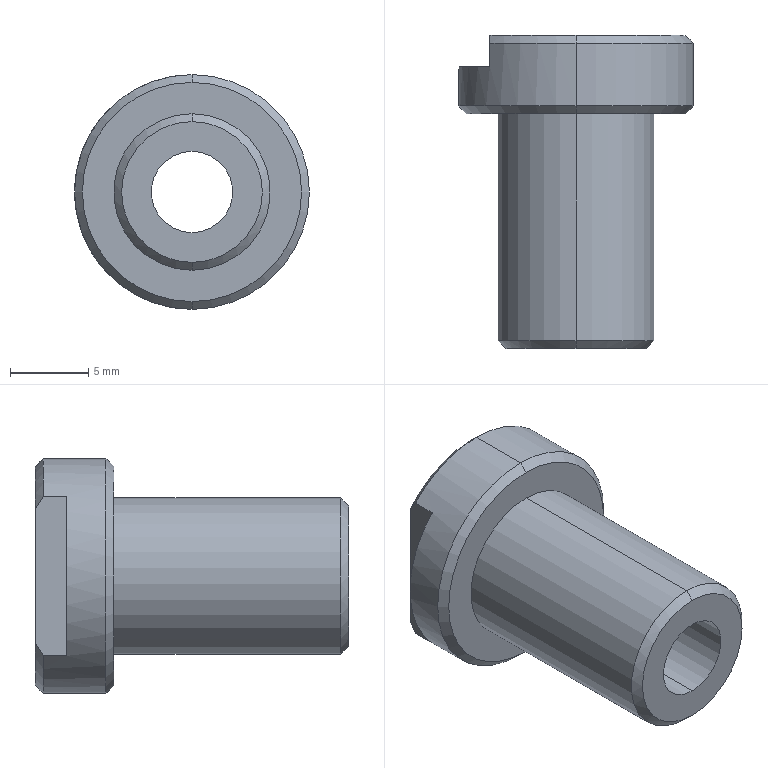Part | SolidWorks | features ICE 2, Chamfer 1, Extrusion 1 | 1 solid | 20 faces | box 15 x 20 x 15 mm | volume 1593 mm3 | cone 9 | cylinder 6 | plane 5 | commonest cylinder face diameters 5.2 x2 10 x2 15 x2
STEP:
#1=CARTESIAN_POINT('',(0.,0.,-4.5));
#2=VERTEX_POINT('',#1);
#3=CARTESIAN_POINT('',(0.,0.,4.5));
#4=VERTEX_POINT('',#3);
#5=CARTESIAN_POINT('',(0.,0.,0.));
#6=DIRECTION('',(0.,-1.,0.));
#7=DIRECTION('',(0.,0.,1.));
#8=AXIS2_PLACEMENT_3D('',#5,#6,#7);
#9=CIRCLE('',#8,4.5);
#10=EDGE_CURVE('',#2,#4,#9,.T.);
#11=ORIENTED_EDGE('',*,*,#10,.F.);
#12=CARTESIAN_POINT('',(0.,0.5,-5.));
#13=VERTEX_POINT('',#12);
#14=CARTESIAN_POINT('',(0.,0.5,-5.));
#15=DIRECTION('',(0.,0.7071,-0.7071));
#16=VECTOR('',#15,1000.);
#17=LINE('',#14,#16);
#18=EDGE_CURVE('',#2,#13,#17,.T.);
#19=ORIENTED_EDGE('',*,*,#18,.T.);
#20=CARTESIAN_POINT('',(0.,0.5,5.));
#21=VERTEX_POINT('',#20);
#22=CARTESIAN_POINT('',(0.,0.5,0.));
#23=DIRECTION('',(0.,1.,0.));
#24=DIRECTION('',(0.,0.,1.));
#25=AXIS2_PLACEMENT_3D('',#22,#23,#24);
#26=CIRCLE('',#25,5.);
#27=EDGE_CURVE('',#21,#13,#26,.T.);
#28=ORIENTED_EDGE('',*,*,#27,.F.);
#29=CARTESIAN_POINT('',(0.,0.5,5.));
#30=DIRECTION('',(0.,0.7071,0.7071));
#31=VECTOR('',#30,1000.);
#32=LINE('',#29,#31);
#33=EDGE_CURVE('',#4,#21,#32,.T.);
#34=ORIENTED_EDGE('',*,*,#33,.F.);
#35=EDGE_LOOP('',(#11,#19,#28,#34));
#36=FACE_OUTER_BOUND('',#35,.T.);
#37=CARTESIAN_POINT('',(0.,0.5,0.));
#38=DIRECTION('',(0.,1.,0.));
#39=DIRECTION('',(0.,0.,1.));
#40=AXIS2_PLACEMENT_3D('',#37,#38,#39);
#41=CONICAL_SURFACE('',#40,5.,0.7854);
#42=ADVANCED_FACE('',(#36),#41,.T.);
#43=CARTESIAN_POINT('',(0.,19.5,-2.6));
#44=VERTEX_POINT('',#43);
#45=CARTESIAN_POINT('',(0.,19.5,2.6));
#46=VERTEX_POINT('',#45);
#47=CARTESIAN_POINT('',(0.,19.5,0.));
#48=DIRECTION('',(0.,1.,0.));
#49=DIRECTION('',(0.,0.,1.));
#50=AXIS2_PLACEMENT_3D('',#47,#48,#49);
#51=CIRCLE('',#50,2.6);
#52=EDGE_CURVE('',#44,#46,#51,.T.);
#53=ORIENTED_EDGE('',*,*,#52,.F.);
#54=CARTESIAN_POINT('',(0.,20.,-3.1));
#55=VERTEX_POINT('',#54);
#56=CARTESIAN_POINT('',(0.,19.5,-2.6));
#57=DIRECTION('',(0.,0.7071,-0.7071));
#58=VECTOR('',#57,1000.);
#59=LINE('',#56,#58);
#60=EDGE_CURVE('',#44,#55,#59,.T.);
#61=ORIENTED_EDGE('',*,*,#60,.T.);
#62=CARTESIAN_POINT('',(0.,20.,3.1));
#63=VERTEX_POINT('',#62);
#64=CARTESIAN_POINT('',(0.,20.,0.));
#65=DIRECTION('',(0.,-1.,0.));
#66=DIRECTION('',(0.,0.,1.));
#67=AXIS2_PLACEMENT_3D('',#64,#65,#66);
#68=CIRCLE('',#67,3.1);
#69=EDGE_CURVE('',#63,#55,#68,.T.);
#70=ORIENTED_EDGE('',*,*,#69,.F.);
#71=CARTESIAN_POINT('',(0.,19.5,2.6));
#72=DIRECTION('',(0.,0.7071,0.7071));
#73=VECTOR('',#72,1000.);
#74=LINE('',#71,#73);
#75=EDGE_CURVE('',#46,#63,#74,.T.);
#76=ORIENTED_EDGE('',*,*,#75,.F.);
#77=EDGE_LOOP('',(#53,#61,#70,#76));
#78=FACE_OUTER_BOUND('',#77,.T.);
#79=CARTESIAN_POINT('',(0.,19.5,0.));
#80=DIRECTION('',(0.,1.,0.));
#81=DIRECTION('',(0.,0.,1.));
#82=AXIS2_PLACEMENT_3D('',#79,#80,#81);
#83=CONICAL_SURFACE('',#82,2.6,0.7854);
#84=ADVANCED_FACE('',(#78),#83,.F.);
#85=CARTESIAN_POINT('',(0.,20.,7.));
#86=VERTEX_POINT('',#85);
#87=CARTESIAN_POINT('',(0.,20.,-7.));
#88=VERTEX_POINT('',#87);
#89=CARTESIAN_POINT('',(0.,20.,0.));
#90=DIRECTION('',(0.,1.,0.));
#91=DIRECTION('',(0.,0.,1.));
#92=AXIS2_PLACEMENT_3D('',#89,#90,#91);
#93=CIRCLE('',#92,7.);
#94=EDGE_CURVE('',#86,#88,#93,.T.);
#95=ORIENTED_EDGE('',*,*,#94,.F.);
#96=CARTESIAN_POINT('',(0.,19.5,7.5));
#97=VERTEX_POINT('',#96);
#98=CARTESIAN_POINT('',(0.,20.,7.));
#99=DIRECTION('',(0.,-0.7071,0.7071));
#100=VECTOR('',#99,1000.);
#101=LINE('',#98,#100);
#102=EDGE_CURVE('',#86,#97,#101,.T.);
#103=ORIENTED_EDGE('',*,*,#102,.T.);
#104=CARTESIAN_POINT('',(0.,19.5,-7.5));
#105=VERTEX_POINT('',#104);
#106=CARTESIAN_POINT('',(0.,19.5,0.));
#107=DIRECTION('',(0.,-1.,0.));
#108=DIRECTION('',(0.,0.,1.));
#109=AXIS2_PLACEMENT_3D('',#106,#107,#108);
#110=CIRCLE('',#109,7.5);
#111=EDGE_CURVE('',#105,#97,#110,.T.);
#112=ORIENTED_EDGE('',*,*,#111,.F.);
#113=CARTESIAN_POINT('',(0.,20.,-7.));
#114=DIRECTION('',(0.,-0.7071,-0.7071));
#115=VECTOR('',#114,1000.);
#116=LINE('',#113,#115);
#117=EDGE_CURVE('',#88,#105,#116,.T.);
#118=ORIENTED_EDGE('',*,*,#117,.F.);
#119=EDGE_LOOP('',(#95,#103,#112,#118));
#120=FACE_OUTER_BOUND('',#119,.T.);
#121=CARTESIAN_POINT('',(0.,20.,0.));
#122=DIRECTION('',(0.,-1.,0.));
#123=DIRECTION('',(0.,0.,-1.));
#124=AXIS2_PLACEMENT_3D('',#121,#122,#123);
#125=CONICAL_SURFACE('',#124,7.,0.7854);
#126=ADVANCED_FACE('',(#120),#125,.T.);
#127=CARTESIAN_POINT('',(-5.5,20.,-4.33));
#128=VERTEX_POINT('',#127);
#129=CARTESIAN_POINT('',(0.,20.,0.));
#130=DIRECTION('',(0.,1.,0.));
#131=DIRECTION('',(0.,0.,1.));
#132=AXIS2_PLACEMENT_3D('',#129,#130,#131);
#133=CIRCLE('',#132,7.);
#134=EDGE_CURVE('',#88,#128,#133,.T.);
#135=ORIENTED_EDGE('',*,*,#134,.F.);
#136=ORIENTED_EDGE('',*,*,#117,.T.);
#137=CARTESIAN_POINT('',(-5.5,19.5,-5.099));
#138=VERTEX_POINT('',#137);
#139=CARTESIAN_POINT('',(0.,19.5,0.));
#140=DIRECTION('',(0.,-1.,0.));
#141=DIRECTION('',(0.,0.,1.));
#142=AXIS2_PLACEMENT_3D('',#139,#140,#141);
#143=CIRCLE('',#142,7.5);
#144=EDGE_CURVE('',#138,#105,#143,.T.);
#145=ORIENTED_EDGE('',*,*,#144,.F.);
#146=CARTESIAN_POINT('',(-5.5,20.,-4.33));
#147=CARTESIAN_POINT('',(-5.5,19.839,-4.59));
#148=CARTESIAN_POINT('',(-5.5,19.672,-4.846));
#149=CARTESIAN_POINT('',(-5.5,19.5,-5.099));
#150=B_SPLINE_CURVE_WITH_KNOTS('',3,(#146,#147,#148,#149),.UNSPECIFIED.,.F.,.F.,(4,4),(0.01014,0.01105),.UNSPECIFIED.);
#151=EDGE_CURVE('',#128,#138,#150,.T.);
#152=ORIENTED_EDGE('',*,*,#151,.F.);
#153=EDGE_LOOP('',(#135,#136,#145,#152));
#154=FACE_OUTER_BOUND('',#153,.T.);
#155=CARTESIAN_POINT('',(0.,20.,0.));
#156=DIRECTION('',(0.,-1.,0.));
#157=DIRECTION('',(0.,0.,-1.));
#158=AXIS2_PLACEMENT_3D('',#155,#156,#157);
#159=CONICAL_SURFACE('',#158,7.,0.7854);
#160=ADVANCED_FACE('',(#154),#159,.T.);
#161=CARTESIAN_POINT('',(0.,15.,-7.));
#162=VERTEX_POINT('',#161);
#163=CARTESIAN_POINT('',(0.,15.,7.));
#164=VERTEX_POINT('',#163);
#165=CARTESIAN_POINT('',(0.,15.,0.));
#166=DIRECTION('',(0.,-1.,0.));
#167=DIRECTION('',(0.,0.,1.));
#168=AXIS2_PLACEMENT_3D('',#165,#166,#167);
#169=CIRCLE('',#168,7.);
#170=EDGE_CURVE('',#162,#164,#169,.T.);
#171=ORIENTED_EDGE('',*,*,#170,.F.);
#172=CARTESIAN_POINT('',(0.,15.5,-7.5));
#173=VERTEX_POINT('',#172);
#174=CARTESIAN_POINT('',(0.,15.5,-7.5));
#175=DIRECTION('',(0.,0.7071,-0.7071));
#176=VECTOR('',#175,1000.);
#177=LINE('',#174,#176);
#178=EDGE_CURVE('',#162,#173,#177,.T.);
#179=ORIENTED_EDGE('',*,*,#178,.T.);
#180=CARTESIAN_POINT('',(0.,15.5,7.5));
#181=VERTEX_POINT('',#180);
#182=CARTESIAN_POINT('',(0.,15.5,0.));
#183=DIRECTION('',(0.,1.,0.));
#184=DIRECTION('',(0.,0.,1.));
#185=AXIS2_PLACEMENT_3D('',#182,#183,#184);
#186=CIRCLE('',#185,7.5);
#187=EDGE_CURVE('',#181,#173,#186,.T.);
#188=ORIENTED_EDGE('',*,*,#187,.F.);
#189=CARTESIAN_POINT('',(0.,15.5,7.5));
#190=DIRECTION('',(0.,0.7071,0.7071));
#191=VECTOR('',#190,1000.);
#192=LINE('',#189,#191);
#193=EDGE_CURVE('',#164,#181,#192,.T.);
#194=ORIENTED_EDGE('',*,*,#193,.F.);
#195=EDGE_LOOP('',(#171,#179,#188,#194));
#196=FACE_OUTER_BOUND('',#195,.T.);
#197=CARTESIAN_POINT('',(0.,15.5,0.));
#198=DIRECTION('',(0.,1.,0.));
#199=DIRECTION('',(0.,0.,1.));
#200=AXIS2_PLACEMENT_3D('',#197,#198,#199);
#201=CONICAL_SURFACE('',#200,7.5,0.7854);
#202=ADVANCED_FACE('',(#196),#201,.T.);
#203=ORIENTED_EDGE('',*,*,#111,.T.);
#204=CARTESIAN_POINT('',(0.,20.,7.5));
#205=DIRECTION('',(0.,-1.,0.));
#206=VECTOR('',#205,1000.);
#207=LINE('',#204,#206);
#208=EDGE_CURVE('',#97,#181,#207,.T.);
#209=ORIENTED_EDGE('',*,*,#208,.T.);
#210=ORIENTED_EDGE('',*,*,#187,.T.);
#211=CARTESIAN_POINT('',(0.,20.,-7.5));
#212=DIRECTION('',(0.,-1.,0.));
#213=VECTOR('',#212,1000.);
#214=LINE('',#211,#213);
#215=EDGE_CURVE('',#105,#173,#214,.T.);
#216=ORIENTED_EDGE('',*,*,#215,.F.);
#217=EDGE_LOOP('',(#203,#209,#210,#216));
#218=FACE_OUTER_BOUND('',#217,.T.);
#219=CARTESIAN_POINT('',(0.,20.,0.));
#220=DIRECTION('',(0.,-1.,0.));
#221=DIRECTION('',(0.,0.,-1.));
#222=AXIS2_PLACEMENT_3D('',#219,#220,#221);
#223=CYLINDRICAL_SURFACE('',#222,7.5);
#224=ADVANCED_FACE('',(#218),#223,.T.);
#225=ORIENTED_EDGE('',*,*,#52,.T.);
#226=CARTESIAN_POINT('',(0.,0.,2.6));
#227=VERTEX_POINT('',#226);
#228=CARTESIAN_POINT('',(0.,15.,2.6));
#229=DIRECTION('',(0.,-1.,0.));
#230=VECTOR('',#229,1000.);
#231=LINE('',#228,#230);
#232=EDGE_CURVE('',#46,#227,#231,.T.);
#233=ORIENTED_EDGE('',*,*,#232,.T.);
#234=CARTESIAN_POINT('',(0.,0.,-2.6));
#235=VERTEX_POINT('',#234);
#236=CARTESIAN_POINT('',(0.,0.,0.));
#237=DIRECTION('',(0.,1.,0.));
#238=DIRECTION('',(0.,0.,1.));
#239=AXIS2_PLACEMENT_3D('',#236,#237,#238);
#240=CIRCLE('',#239,2.6);
#241=EDGE_CURVE('',#235,#227,#240,.T.);
#242=ORIENTED_EDGE('',*,*,#241,.F.);
#243=CARTESIAN_POINT('',(0.,15.,-2.6));
#244=DIRECTION('',(0.,-1.,0.));
#245=VECTOR('',#244,1000.);
#246=LINE('',#243,#245);
#247=EDGE_CURVE('',#44,#235,#246,.T.);
#248=ORIENTED_EDGE('',*,*,#247,.F.);
#249=EDGE_LOOP('',(#225,#233,#242,#248));
#250=FACE_OUTER_BOUND('',#249,.T.);
#251=CARTESIAN_POINT('',(0.,15.,0.));
#252=DIRECTION('',(0.,-1.,0.));
#253=DIRECTION('',(0.,0.,-1.));
#254=AXIS2_PLACEMENT_3D('',#251,#252,#253);
#255=CYLINDRICAL_SURFACE('',#254,2.6);
#256=ADVANCED_FACE('',(#250),#255,.F.);
#257=CARTESIAN_POINT('',(0.,15.,5.));
#258=VERTEX_POINT('',#257);
#259=CARTESIAN_POINT('',(0.,15.,-5.));
#260=VERTEX_POINT('',#259);
#261=CARTESIAN_POINT('',(0.,15.,0.));
#262=DIRECTION('',(0.,1.,0.));
#263=DIRECTION('',(0.,0.,1.));
#264=AXIS2_PLACEMENT_3D('',#261,#262,#263);
#265=CIRCLE('',#264,5.);
#266=EDGE_CURVE('',#258,#260,#265,.T.);
#267=ORIENTED_EDGE('',*,*,#266,.F.);
#268=CARTESIAN_POINT('',(0.,15.,5.));
#269=DIRECTION('',(0.,-1.,0.));
#270=VECTOR('',#269,1000.);
#271=LINE('',#268,#270);
#272=EDGE_CURVE('',#258,#21,#271,.T.);
#273=ORIENTED_EDGE('',*,*,#272,.T.);
#274=ORIENTED_EDGE('',*,*,#27,.T.);
#275=CARTESIAN_POINT('',(0.,15.,-5.));
#276=DIRECTION('',(0.,-1.,0.));
#277=VECTOR('',#276,1000.);
#278=LINE('',#275,#277);
#279=EDGE_CURVE('',#260,#13,#278,.T.);
#280=ORIENTED_EDGE('',*,*,#279,.F.);
#281=EDGE_LOOP('',(#267,#273,#274,#280));
#282=FACE_OUTER_BOUND('',#281,.T.);
#283=CARTESIAN_POINT('',(0.,15.,0.));
#284=DIRECTION('',(0.,-1.,0.));
#285=DIRECTION('',(0.,0.,-1.));
#286=AXIS2_PLACEMENT_3D('',#283,#284,#285);
#287=CYLINDRICAL_SURFACE('',#286,5.);
#288=ADVANCED_FACE('',(#282),#287,.T.);
#289=CARTESIAN_POINT('',(0.,0.,0.));
#290=DIRECTION('',(0.,-1.,0.));
#291=DIRECTION('',(0.,0.,1.));
#292=AXIS2_PLACEMENT_3D('',#289,#290,#291);
#293=CIRCLE('',#292,4.5);
#294=EDGE_CURVE('',#4,#2,#293,.T.);
#295=ORIENTED_EDGE('',*,*,#294,.T.);
#296=ORIENTED_EDGE('',*,*,#10,.T.);
#297=EDGE_LOOP('',(#295,#296));
#298=FACE_OUTER_BOUND('',#297,.T.);
#299=ORIENTED_EDGE('',*,*,#241,.T.);
#300=CARTESIAN_POINT('',(0.,0.,0.));
#301=DIRECTION('',(0.,1.,0.));
#302=DIRECTION('',(0.,0.,1.));
#303=AXIS2_PLACEMENT_3D('',#300,#301,#302);
#304=CIRCLE('',#303,2.6);
#305=EDGE_CURVE('',#227,#235,#304,.T.);
#306=ORIENTED_EDGE('',*,*,#305,.T.);
#307=EDGE_LOOP('',(#299,#306));
#308=FACE_BOUND('',#307,.T.);
#309=CARTESIAN_POINT('',(0.,0.,0.));
#310=DIRECTION('',(0.,1.,0.));
#311=DIRECTION('',(0.,0.,1.));
#312=AXIS2_PLACEMENT_3D('',#309,#310,#311);
#313=PLANE('',#312);
#314=ADVANCED_FACE('',(#298,#308),#313,.F.);
#315=ORIENTED_EDGE('',*,*,#272,.F.);
#316=CARTESIAN_POINT('',(0.,15.,0.));
#317=DIRECTION('',(0.,1.,0.));
#318=DIRECTION('',(0.,0.,1.));
#319=AXIS2_PLACEMENT_3D('',#316,#317,#318);
#320=CIRCLE('',#319,5.);
#321=EDGE_CURVE('',#260,#258,#320,.T.);
#322=ORIENTED_EDGE('',*,*,#321,.F.);
#323=ORIENTED_EDGE('',*,*,#279,.T.);
#324=CARTESIAN_POINT('',(0.,0.5,0.));
#325=DIRECTION('',(0.,1.,0.));
#326=DIRECTION('',(0.,0.,1.));
#327=AXIS2_PLACEMENT_3D('',#324,#325,#326);
#328=CIRCLE('',#327,5.);
#329=EDGE_CURVE('',#13,#21,#328,.T.);
#330=ORIENTED_EDGE('',*,*,#329,.T.);
#331=EDGE_LOOP('',(#315,#322,#323,#330));
#332=FACE_OUTER_BOUND('',#331,.T.);
#333=CARTESIAN_POINT('',(0.,15.,0.));
#334=DIRECTION('',(0.,-1.,0.));
#335=DIRECTION('',(0.,0.,-1.));
#336=AXIS2_PLACEMENT_3D('',#333,#334,#335);
#337=CYLINDRICAL_SURFACE('',#336,5.);
#338=ADVANCED_FACE('',(#332),#337,.T.);
#339=ORIENTED_EDGE('',*,*,#232,.F.);
#340=CARTESIAN_POINT('',(0.,19.5,0.));
#341=DIRECTION('',(0.,1.,0.));
#342=DIRECTION('',(0.,0.,1.));
#343=AXIS2_PLACEMENT_3D('',#340,#341,#342);
#344=CIRCLE('',#343,2.6);
#345=EDGE_CURVE('',#46,#44,#344,.T.);
#346=ORIENTED_EDGE('',*,*,#345,.T.);
#347=ORIENTED_EDGE('',*,*,#247,.T.);
#348=ORIENTED_EDGE('',*,*,#305,.F.);
#349=EDGE_LOOP('',(#339,#346,#347,#348));
#350=FACE_OUTER_BOUND('',#349,.T.);
#351=CARTESIAN_POINT('',(0.,15.,0.));
#352=DIRECTION('',(0.,-1.,0.));
#353=DIRECTION('',(0.,0.,-1.));
#354=AXIS2_PLACEMENT_3D('',#351,#352,#353);
#355=CYLINDRICAL_SURFACE('',#354,2.6);
#356=ADVANCED_FACE('',(#350),#355,.F.);
#357=CARTESIAN_POINT('',(-5.5,20.,4.33));
#358=VERTEX_POINT('',#357);
#359=CARTESIAN_POINT('',(-5.5,20.,0.));
#360=DIRECTION('',(0.,0.,-1.));
#361=VECTOR('',#360,1000.);
#362=LINE('',#359,#361);
#363=EDGE_CURVE('',#358,#128,#362,.T.);
#364=ORIENTED_EDGE('',*,*,#363,.F.);
#365=CARTESIAN_POINT('',(0.,20.,0.));
#366=DIRECTION('',(0.,1.,0.));
#367=DIRECTION('',(0.,0.,1.));
#368=AXIS2_PLACEMENT_3D('',#365,#366,#367);
#369=CIRCLE('',#368,7.);
#370=EDGE_CURVE('',#358,#86,#369,.T.);
#371=ORIENTED_EDGE('',*,*,#370,.T.);
#372=ORIENTED_EDGE('',*,*,#94,.T.);
#373=ORIENTED_EDGE('',*,*,#134,.T.);
#374=EDGE_LOOP('',(#364,#371,#372,#373));
#375=FACE_OUTER_BOUND('',#374,.T.);
#376=ORIENTED_EDGE('',*,*,#69,.T.);
#377=CARTESIAN_POINT('',(0.,20.,0.));
#378=DIRECTION('',(0.,-1.,0.));
#379=DIRECTION('',(0.,0.,1.));
#380=AXIS2_PLACEMENT_3D('',#377,#378,#379);
#381=CIRCLE('',#380,3.1);
#382=EDGE_CURVE('',#55,#63,#381,.T.);
#383=ORIENTED_EDGE('',*,*,#382,.T.);
#384=EDGE_LOOP('',(#376,#383));
#385=FACE_BOUND('',#384,.T.);
#386=CARTESIAN_POINT('',(0.,20.,0.));
#387=DIRECTION('',(0.,1.,0.));
#388=DIRECTION('',(0.,0.,1.));
#389=AXIS2_PLACEMENT_3D('',#386,#387,#388);
#390=PLANE('',#389);
#391=ADVANCED_FACE('',(#375,#385),#390,.T.);
#392=CARTESIAN_POINT('',(0.,15.,0.));
#393=DIRECTION('',(0.,-1.,0.));
#394=DIRECTION('',(0.,0.,1.));
#395=AXIS2_PLACEMENT_3D('',#392,#393,#394);
#396=CIRCLE('',#395,7.);
#397=EDGE_CURVE('',#164,#162,#396,.T.);
#398=ORIENTED_EDGE('',*,*,#397,.T.);
#399=ORIENTED_EDGE('',*,*,#170,.T.);
#400=EDGE_LOOP('',(#398,#399));
#401=FACE_OUTER_BOUND('',#400,.T.);
#402=ORIENTED_EDGE('',*,*,#321,.T.);
#403=ORIENTED_EDGE('',*,*,#266,.T.);
#404=EDGE_LOOP('',(#402,#403));
#405=FACE_BOUND('',#404,.T.);
#406=CARTESIAN_POINT('',(0.,15.,0.));
#407=DIRECTION('',(0.,1.,0.));
#408=DIRECTION('',(0.,0.,1.));
#409=AXIS2_PLACEMENT_3D('',#406,#407,#408);
#410=PLANE('',#409);
#411=ADVANCED_FACE('',(#401,#405),#410,.F.);
#412=ORIENTED_EDGE('',*,*,#208,.F.);
#413=CARTESIAN_POINT('',(-5.5,19.5,5.099));
#414=VERTEX_POINT('',#413);
#415=CARTESIAN_POINT('',(0.,19.5,0.));
#416=DIRECTION('',(0.,-1.,0.));
#417=DIRECTION('',(0.,0.,1.));
#418=AXIS2_PLACEMENT_3D('',#415,#416,#417);
#419=CIRCLE('',#418,7.5);
#420=EDGE_CURVE('',#97,#414,#419,.T.);
#421=ORIENTED_EDGE('',*,*,#420,.T.);
#422=CARTESIAN_POINT('',(-5.5,18.,5.099));
#423=VERTEX_POINT('',#422);
#424=CARTESIAN_POINT('',(-5.5,20.,5.099));
#425=DIRECTION('',(0.,-1.,0.));
#426=VECTOR('',#425,1000.);
#427=LINE('',#424,#426);
#428=EDGE_CURVE('',#414,#423,#427,.T.);
#429=ORIENTED_EDGE('',*,*,#428,.T.);
#430=CARTESIAN_POINT('',(-5.5,18.,-5.099));
#431=VERTEX_POINT('',#430);
#432=CARTESIAN_POINT('',(0.,18.,0.));
#433=DIRECTION('',(0.,-1.,0.));
#434=DIRECTION('',(0.,0.,-1.));
#435=AXIS2_PLACEMENT_3D('',#432,#433,#434);
#436=CIRCLE('',#435,7.5);
#437=EDGE_CURVE('',#423,#431,#436,.T.);
#438=ORIENTED_EDGE('',*,*,#437,.T.);
#439=CARTESIAN_POINT('',(-5.5,20.,-5.099));
#440=DIRECTION('',(0.,1.,0.));
#441=VECTOR('',#440,1000.);
#442=LINE('',#439,#441);
#443=EDGE_CURVE('',#431,#138,#442,.T.);
#444=ORIENTED_EDGE('',*,*,#443,.T.);
#445=ORIENTED_EDGE('',*,*,#144,.T.);
#446=ORIENTED_EDGE('',*,*,#215,.T.);
#447=CARTESIAN_POINT('',(0.,15.5,0.));
#448=DIRECTION('',(0.,1.,0.));
#449=DIRECTION('',(0.,0.,1.));
#450=AXIS2_PLACEMENT_3D('',#447,#448,#449);
#451=CIRCLE('',#450,7.5);
#452=EDGE_CURVE('',#173,#181,#451,.T.);
#453=ORIENTED_EDGE('',*,*,#452,.T.);
#454=EDGE_LOOP('',(#412,#421,#429,#438,#444,#445,#446,#453));
#455=FACE_OUTER_BOUND('',#454,.T.);
#456=CARTESIAN_POINT('',(0.,20.,0.));
#457=DIRECTION('',(0.,-1.,0.));
#458=DIRECTION('',(0.,0.,-1.));
#459=AXIS2_PLACEMENT_3D('',#456,#457,#458);
#460=CYLINDRICAL_SURFACE('',#459,7.5);
#461=ADVANCED_FACE('',(#455),#460,.T.);
#462=ORIENTED_EDGE('',*,*,#178,.F.);
#463=ORIENTED_EDGE('',*,*,#397,.F.);
#464=ORIENTED_EDGE('',*,*,#193,.T.);
#465=ORIENTED_EDGE('',*,*,#452,.F.);
#466=EDGE_LOOP('',(#462,#463,#464,#465));
#467=FACE_OUTER_BOUND('',#466,.T.);
#468=CARTESIAN_POINT('',(0.,15.5,0.));
#469=DIRECTION('',(0.,1.,0.));
#470=DIRECTION('',(0.,0.,1.));
#471=AXIS2_PLACEMENT_3D('',#468,#469,#470);
#472=CONICAL_SURFACE('',#471,7.5,0.7854);
#473=ADVANCED_FACE('',(#467),#472,.T.);
#474=ORIENTED_EDGE('',*,*,#102,.F.);
#475=ORIENTED_EDGE('',*,*,#370,.F.);
#476=CARTESIAN_POINT('',(-5.5,19.5,5.099));
#477=CARTESIAN_POINT('',(-5.5,19.672,4.846));
#478=CARTESIAN_POINT('',(-5.5,19.839,4.59));
#479=CARTESIAN_POINT('',(-5.5,20.,4.33));
#480=B_SPLINE_CURVE_WITH_KNOTS('',3,(#476,#477,#478,#479),.UNSPECIFIED.,.F.,.F.,(4,4),(0.000001236,0.0009141),.UNSPECIFIED.);
#481=EDGE_CURVE('',#414,#358,#480,.T.);
#482=ORIENTED_EDGE('',*,*,#481,.F.);
#483=ORIENTED_EDGE('',*,*,#420,.F.);
#484=EDGE_LOOP('',(#474,#475,#482,#483));
#485=FACE_OUTER_BOUND('',#484,.T.);
#486=CARTESIAN_POINT('',(0.,20.,0.));
#487=DIRECTION('',(0.,-1.,0.));
#488=DIRECTION('',(0.,0.,-1.));
#489=AXIS2_PLACEMENT_3D('',#486,#487,#488);
#490=CONICAL_SURFACE('',#489,7.,0.7854);
#491=ADVANCED_FACE('',(#485),#490,.T.);
#492=ORIENTED_EDGE('',*,*,#60,.F.);
#493=ORIENTED_EDGE('',*,*,#345,.F.);
#494=ORIENTED_EDGE('',*,*,#75,.T.);
#495=ORIENTED_EDGE('',*,*,#382,.F.);
#496=EDGE_LOOP('',(#492,#493,#494,#495));
#497=FACE_OUTER_BOUND('',#496,.T.);
#498=CARTESIAN_POINT('',(0.,19.5,0.));
#499=DIRECTION('',(0.,1.,0.));
#500=DIRECTION('',(0.,0.,1.));
#501=AXIS2_PLACEMENT_3D('',#498,#499,#500);
#502=CONICAL_SURFACE('',#501,2.6,0.7854);
#503=ADVANCED_FACE('',(#497),#502,.F.);
#504=ORIENTED_EDGE('',*,*,#18,.F.);
#505=ORIENTED_EDGE('',*,*,#294,.F.);
#506=ORIENTED_EDGE('',*,*,#33,.T.);
#507=ORIENTED_EDGE('',*,*,#329,.F.);
#508=EDGE_LOOP('',(#504,#505,#506,#507));
#509=FACE_OUTER_BOUND('',#508,.T.);
#510=CARTESIAN_POINT('',(0.,0.5,0.));
#511=DIRECTION('',(0.,1.,0.));
#512=DIRECTION('',(0.,0.,1.));
#513=AXIS2_PLACEMENT_3D('',#510,#511,#512);
#514=CONICAL_SURFACE('',#513,5.,0.7854);
#515=ADVANCED_FACE('',(#509),#514,.T.);
#516=CARTESIAN_POINT('',(-5.5,18.,-25.));
#517=DIRECTION('',(0.,0.,1.));
#518=VECTOR('',#517,1000.);
#519=LINE('',#516,#518);
#520=EDGE_CURVE('',#431,#423,#519,.T.);
#521=ORIENTED_EDGE('',*,*,#520,.F.);
#522=ORIENTED_EDGE('',*,*,#437,.F.);
#523=EDGE_LOOP('',(#521,#522));
#524=FACE_OUTER_BOUND('',#523,.T.);
#525=CARTESIAN_POINT('',(-10.5,18.,-25.));
#526=DIRECTION('',(0.,-1.,0.));
#527=DIRECTION('',(0.,0.,-1.));
#528=AXIS2_PLACEMENT_3D('',#525,#526,#527);
#529=PLANE('',#528);
#530=ADVANCED_FACE('',(#524),#529,.F.);
#531=ORIENTED_EDGE('',*,*,#481,.T.);
#532=ORIENTED_EDGE('',*,*,#363,.T.);
#533=ORIENTED_EDGE('',*,*,#151,.T.);
#534=ORIENTED_EDGE('',*,*,#443,.F.);
#535=ORIENTED_EDGE('',*,*,#520,.T.);
#536=ORIENTED_EDGE('',*,*,#428,.F.);
#537=EDGE_LOOP('',(#531,#532,#533,#534,#535,#536));
#538=FACE_OUTER_BOUND('',#537,.T.);
#539=CARTESIAN_POINT('',(-5.5,23.,-25.));
#540=DIRECTION('',(1.,0.,0.));
#541=DIRECTION('',(0.,1.,0.));
#542=AXIS2_PLACEMENT_3D('',#539,#540,#541);
#543=PLANE('',#542);
#544=ADVANCED_FACE('',(#538),#543,.F.);
#545=CLOSED_SHELL('',(#42,#84,#126,#160,#202,#224,#256,#288,#314,#338,#356,#391,#411,#461,#473,#491,#503,#515,#530,#544));
#546=MANIFOLD_SOLID_BREP('',#545);
#547=CARTESIAN_POINT('',(0.,0.,0.));
#548=DIRECTION('',(0.,0.,1.));
#549=DIRECTION('',(1.,0.,0.));
#550=AXIS2_PLACEMENT_3D('',#547,#548,#549);
#551=(LENGTH_UNIT()NAMED_UNIT(*)SI_UNIT(.MILLI.,.METRE.));
#552=UNCERTAINTY_MEASURE_WITH_UNIT(LENGTH_MEASURE(0.00001),#551,'','');
#553=(NAMED_UNIT(*)PLANE_ANGLE_UNIT()SI_UNIT($,.RADIAN.));
#554=(NAMED_UNIT(*)SI_UNIT($,.STERADIAN.)SOLID_ANGLE_UNIT());
#555=(GEOMETRIC_REPRESENTATION_CONTEXT(3)GLOBAL_UNCERTAINTY_ASSIGNED_CONTEXT((#552))GLOBAL_UNIT_ASSIGNED_CONTEXT((#551,#553,#554))REPRESENTATION_CONTEXT('',''));
#556=ADVANCED_BREP_SHAPE_REPRESENTATION('',(#546,#550),#555);